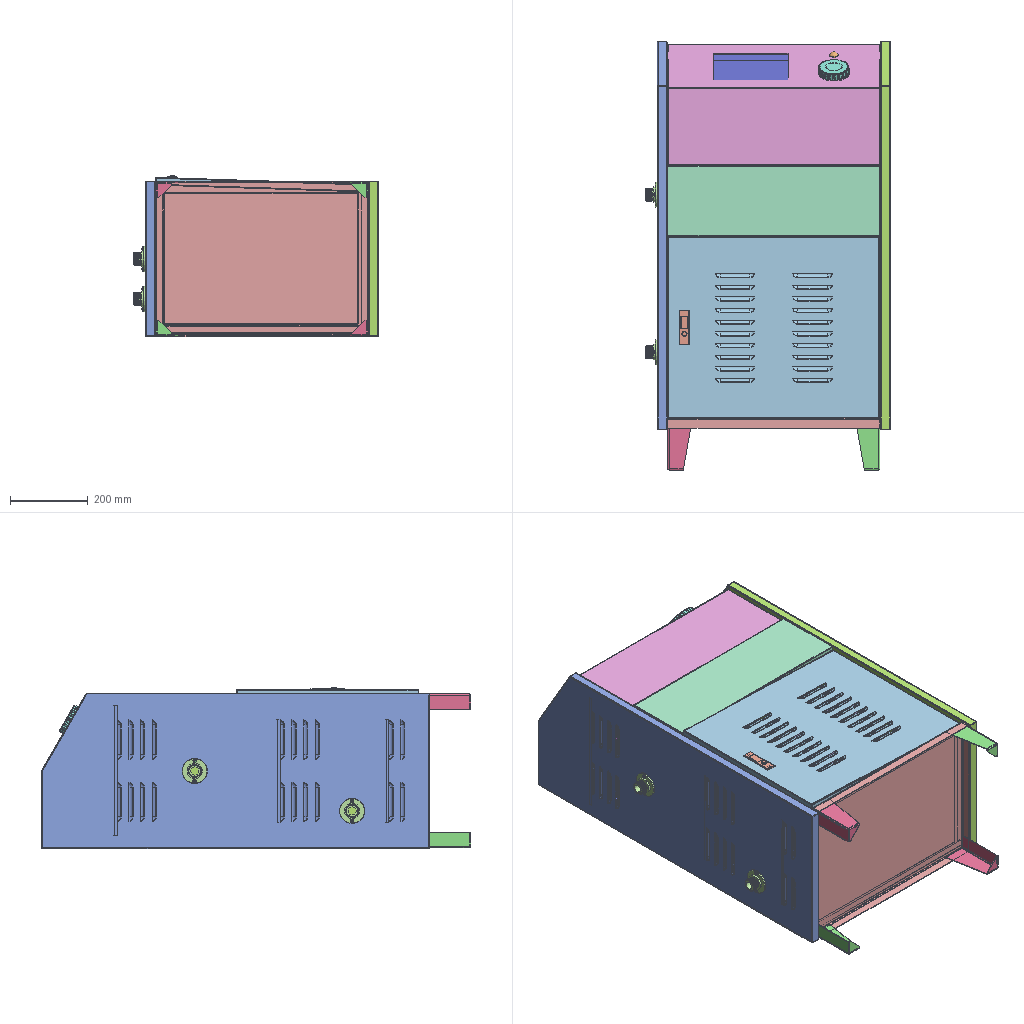Assembly | SolidWorks | 19 different items | 23 placed | box 630 x 1105 x 415 mm
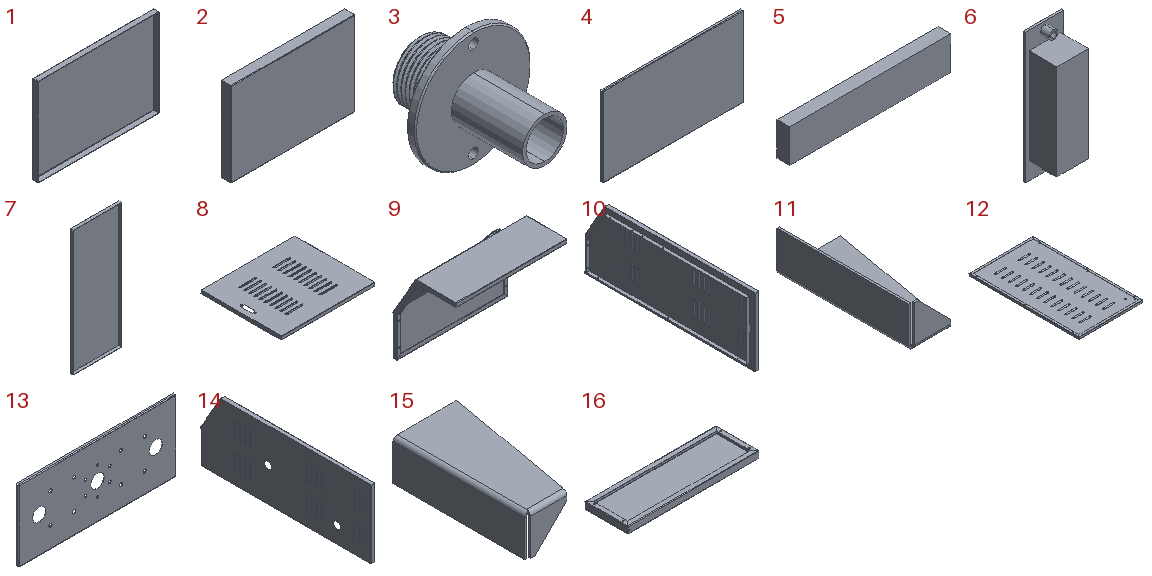Parts list (item | name | quantity | size | volume | features):
1 | - | x1 | 550 x 25 x 400 mm | 521630 mm3 | features Cut 1, EdgeFlange 1, FlatPattern 1, SMBaseFlange 1, SheetMetal 1
2 | - | x1 | 500 x 40 x 340 mm | 280304 mm3 | features EdgeFlange 1, FlatPattern 1, SMBaseFlange 1, SheetMetal 1
3 | - | x2 | 65 x 70 x 65 mm | 33296 mm3 | features Helix 1, ICE 1, Revolution 1, SweepCut 1
4 | - | x1 | 596 x 10 x 338 mm | 259798 mm3 | features EdgeFlange 1, FlatPattern 1, SMBaseFlange 1, SheetMetal 1
5 | - | x1 | 151.025 x 16 x 31.377 mm | 59353 mm3 | features Fillet 2, Extrusion 1, FormToolCreator 1, ICE 1
6 | - | x1 | 26 x 25 x 89 mm | 33780 mm3 | features ICE 2, BossThin 1, Chamfer 1, CutThin 1, Extrusion 1, Fillet 1
7 | - | x1 | 270 x 16.5 x 695 mm | 322735 mm3 | features EdgeFlange 1, FlatPattern 1, SMBaseFlange 1, SheetMetal 1
8 | - | x1 | 546 x 468 x 20 mm | 392970 mm3 | features EdgeFlange 2, Cut 1, FlatPattern 1, FormToolInstance 1, ICE 1, SMBaseFlange 1, SheetMetal 1
9 | - | x1 | 549 x 311.751 x 391.2 mm | 563037 mm3 | features ICE 9, EdgeFlange 2, Fillet 2, CirPattern 1, Dome 1, FlatPattern 1, Fold 1, SMBaseFlange 1, SheetMetal 1, UnFold 1
10 | - | x1 | 43.8 x 1000 x 400 mm | 684379 mm3 | features Cut 3, EdgeFlange 3, FormToolInstance 3, ICE 2, FlatPattern 1, Fold 1, SMBaseFlange 1, SheetMetal 1, UnFold 1
11 | - | x2 | 62.923 x 132 x 40 mm | 24687 mm3 | features Chamfer 1, EdgeFlange 1, Extrusion 1, FlatPattern 1, ICE 1, MirrorSolid 1, SheetMetal 1, Shell 1, SolidToSheetMetal 1
12 | - | x1 | 548 x 940 x 20 mm | 744289 mm3 | features EdgeFlange 2, FlatPattern 1, FormToolInstance 1, ICE 1, SMBaseFlange 1, SheetMetal 1
13 | - | x2 | 596 x 10 x 270 mm | 331666 mm3 | features EdgeFlange 1, FlatPattern 1, ICE 1, SMBaseFlange 1, SheetMetal 1
14 | - | x1 | 43.8 x 1000 x 400 mm | 681227 mm3 | features Cut 4, EdgeFlange 3, FormToolInstance 3, ICE 2, FlatPattern 1, Fold 1, SMBaseFlange 1, SheetMetal 1, UnFold 1
15 | - | x2 | 62.923 x 132 x 40 mm | 24687 mm3 | features Chamfer 1, EdgeFlange 1, Extrusion 1, FlatPattern 1, SheetMetal 1, Shell 1, SolidToSheetMetal 1
16 | - | x1 | 550 x 180 x 28.8 mm | 193683 mm3 | features EdgeFlange 2, Cut 1, FlatPattern 1, ICE 1, SMBaseFlange 1, SheetMetal 1
17 | hex nuts 1-fine pitch-grades ab gb | x1 | - | - | -
18 | hex screw gradeab fine_din | x1 | - | - | -
19 | pan head cross recess screw_din | x1 | - | - | -
Mates (type | each side: item.copy, entity, surface, feature):
DistanceDim | 9.1 face plane Edge-Flange1 | 10.1 face plane Edge-Flange2
Coincident | 10.1 face plane Edge-Flange1 | 9.1 face plane Edge-Flange1
Coincident | 10.1 face plane Edge-Flange6 | 9.1 face plane Edge-Flange2
Coincident | 14.1 face plane Edge-Flange7 | 9.1 face plane Edge-Flange2
DistanceDim | 14.1 face plane Edge-Flange2 | 9.1 face plane Edge-Flange1
Coincident | 14.1 face plane Edge-Flange1 | 9.1 face plane Edge-Flange1
Coincident | 1.1 face plane Base-Flange1 | 14.1 face plane Edge-Flange7
Coincident | 1.1 face plane Edge-Flange1 | 14.1 face plane Edge-Flange2
Coincident | 1.1 face plane Edge-Flange1 | 14.1 face plane Edge-Flange1
Coincident | 14.1 face plane Edge-Flange7 | 16.1 face plane Edge-Flange2
DistanceDim | 16.1 face plane Edge-Flange1 | 9.1 face plane Edge-Flange1
Coincident | 1.1 face plane Base-Flange1 | 8.1 face plane Edge-Flange1
Coincident | 14.1 face plane Edge-Flange2 | 16.1 face plane Edge-Flange1
Concentric | 1.1 face cylinder Cut-Extrude1 | 8.1 face cylinder Cut-Extrude1
DistanceDim | 13.1 face plane Edge-Flange1 | 10.1 face plane Base-Flange1
DistanceDim | 13.2 face plane Edge-Flange1 | 10.1 face plane Base-Flange1
Coincident | 10.1 edge | 13.2 face plane Edge-Flange1
DistanceDim | 10.1 edge | 13.2 edge
DistanceDim | 4.1 face plane Edge-Flange1 | 10.1 face plane Base-Flange1
DistanceDim | 4.1 face plane Edge-Flange1 | 10.1 face plane Edge-Flange6
Coincident | 10.1 edge | 4.1 face plane Edge-Flange1
Coincident | 10.1 edge | 13.1 face plane Edge-Flange1
Coincident | 1.1 face plane Base-Flange1 | 2.1 face plane Base-Flange1
Coincident | 14.1 face plane Edge-Flange7 | 2.1 face plane Edge-Flange1
DistanceDim | 14.1 face plane Edge-Flange7 | 2.1 face plane Edge-Flange1
Coincident | 10.1 face plane Edge-Flange6 | 12.1 face plane Edge-Flange2
DistanceDim | 12.1 face plane Edge-Flange1 | 10.1 face plane Edge-Flange2
Coincident | 1.1 face plane Base-Flange1 | 12.1 face plane Edge-Flange1
Coincident | 11.1 face plane Mirror1 | 15.1 face plane Convert Entities1
Coincident | 11.2 face plane Mirror1 | 15.1 face plane Convert Entities1
Coincident | 11.2 face plane Mirror1 | 15.2 face plane Convert Entities1
Coincident | 1.1 face plane Base-Flange1 | 15.2 face plane Convert Entities1
Coincident | 1.1 face plane Edge-Flange1 | 11.2 face plane Mirror1
Coincident | 1.1 face plane Edge-Flange1 | 11.2 face plane Convert Entities1
Coincident | 1.1 face plane Edge-Flange1 | 15.2 face plane Convert Entities1 | 2 times
Coincident | 1.1 face plane Edge-Flange1 | 11.1 face plane Mirror1
Coincident | 1.1 face plane Edge-Flange1 | 11.1 face plane Convert Entities1
Coincident | 1.1 face plane Edge-Flange1 | 15.1 face plane Convert Entities1 | 2 times
Coincident | 8.1 face plane Base-Flange1 | 6.1 face plane Boss-Extrude1
Concentric | 14.1 edge | 3.1 face cylinder Revolve1
Concentric | 14.1 edge | 3.2 face cylinder Revolve1
Coincident | 14.1 face plane Base-Flange1 | 3.1 face plane Revolve1
Coincident | 14.1 face plane Base-Flange1 | 3.2 face plane Revolve1
Concentric | 14.1 edge | 3.2 edge
Concentric | 14.1 edge | 3.1 edge
Concentric | 8.1 edge | 6.1 edge